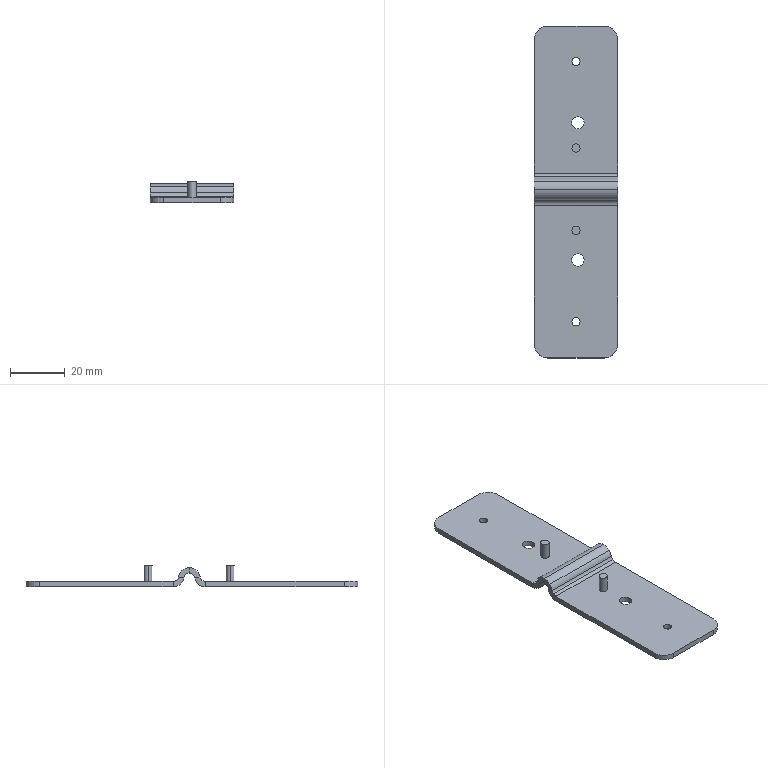Part | NX | features BREP 1 | 1 solid | 48 faces | box 30.5 x 121 x 8 mm | volume 7636 mm3 | cylinder 28 | plane 20 | commonest cylinder face diameters 3 x8 4 x6 8 x6 4.5 x4 10 x4
STEP:
#1=CARTESIAN_POINT('',(94.764,92.,225.465));
#2=VERTEX_POINT('',#1);
#3=CARTESIAN_POINT('',(97.764,92.,225.465));
#4=VERTEX_POINT('',#3);
#5=CARTESIAN_POINT('',(96.264,92.,225.465));
#6=DIRECTION('',(0.,0.,1.));
#7=DIRECTION('',(1.,0.,0.));
#8=AXIS2_PLACEMENT_3D('',#5,#6,#7);
#9=CIRCLE('',#8,1.5);
#10=EDGE_CURVE('',#2,#4,#9,.T.);
#11=ORIENTED_EDGE('',*,*,#10,.T.);
#12=CARTESIAN_POINT('',(96.264,92.,225.465));
#13=DIRECTION('',(0.,0.,1.));
#14=DIRECTION('',(1.,0.,0.));
#15=AXIS2_PLACEMENT_3D('',#12,#13,#14);
#16=CIRCLE('',#15,1.5);
#17=EDGE_CURVE('',#4,#2,#16,.T.);
#18=ORIENTED_EDGE('',*,*,#17,.T.);
#19=EDGE_LOOP('',(#11,#18));
#20=FACE_BOUND('',#19,.T.);
#21=CARTESIAN_POINT('',(0.,0.,225.465));
#22=DIRECTION('',(0.,0.,1.));
#23=DIRECTION('',(1.,0.,0.));
#24=AXIS2_PLACEMENT_3D('',#21,#22,#23);
#25=PLANE('',#24);
#26=ADVANCED_FACE('',(#20),#25,.T.);
#27=CARTESIAN_POINT('',(94.764,92.,219.465));
#28=VERTEX_POINT('',#27);
#29=CARTESIAN_POINT('',(94.764,92.,222.465));
#30=DIRECTION('',(0.,0.,-1.));
#31=VECTOR('',#30,1000.);
#32=LINE('',#29,#31);
#33=EDGE_CURVE('',#2,#28,#32,.T.);
#34=ORIENTED_EDGE('',*,*,#33,.T.);
#35=CARTESIAN_POINT('',(97.764,92.,219.465));
#36=VERTEX_POINT('',#35);
#37=CARTESIAN_POINT('',(96.264,92.,219.465));
#38=DIRECTION('',(0.,0.,1.));
#39=DIRECTION('',(1.,0.,0.));
#40=AXIS2_PLACEMENT_3D('',#37,#38,#39);
#41=CIRCLE('',#40,1.5);
#42=EDGE_CURVE('',#28,#36,#41,.T.);
#43=ORIENTED_EDGE('',*,*,#42,.T.);
#44=CARTESIAN_POINT('',(97.764,92.,222.465));
#45=DIRECTION('',(0.,0.,-1.));
#46=VECTOR('',#45,1000.);
#47=LINE('',#44,#46);
#48=EDGE_CURVE('',#4,#36,#47,.T.);
#49=ORIENTED_EDGE('',*,*,#48,.F.);
#50=ORIENTED_EDGE('',*,*,#10,.F.);
#51=EDGE_LOOP('',(#34,#43,#49,#50));
#52=FACE_BOUND('',#51,.T.);
#53=CARTESIAN_POINT('',(96.264,92.,222.465));
#54=DIRECTION('',(0.,0.,1.));
#55=DIRECTION('',(-1.,0.,0.));
#56=AXIS2_PLACEMENT_3D('',#53,#54,#55);
#57=CYLINDRICAL_SURFACE('',#56,1.5);
#58=ADVANCED_FACE('',(#52),#57,.T.);
#59=ORIENTED_EDGE('',*,*,#48,.T.);
#60=CARTESIAN_POINT('',(96.264,92.,219.465));
#61=DIRECTION('',(0.,0.,1.));
#62=DIRECTION('',(1.,0.,0.));
#63=AXIS2_PLACEMENT_3D('',#60,#61,#62);
#64=CIRCLE('',#63,1.5);
#65=EDGE_CURVE('',#36,#28,#64,.T.);
#66=ORIENTED_EDGE('',*,*,#65,.T.);
#67=ORIENTED_EDGE('',*,*,#33,.F.);
#68=ORIENTED_EDGE('',*,*,#17,.F.);
#69=EDGE_LOOP('',(#59,#66,#67,#68));
#70=FACE_BOUND('',#69,.T.);
#71=CARTESIAN_POINT('',(96.264,92.,222.465));
#72=DIRECTION('',(0.,0.,1.));
#73=DIRECTION('',(-1.,0.,0.));
#74=AXIS2_PLACEMENT_3D('',#71,#72,#73);
#75=CYLINDRICAL_SURFACE('',#74,1.5);
#76=ADVANCED_FACE('',(#70),#75,.T.);
#77=CARTESIAN_POINT('',(94.689,81.216,217.465));
#78=VERTEX_POINT('',#77);
#79=CARTESIAN_POINT('',(94.689,81.216,219.465));
#80=VERTEX_POINT('',#79);
#81=CARTESIAN_POINT('',(94.689,81.216,217.465));
#82=DIRECTION('',(0.,0.,1.));
#83=VECTOR('',#82,1000.);
#84=LINE('',#81,#83);
#85=EDGE_CURVE('',#78,#80,#84,.T.);
#86=ORIENTED_EDGE('',*,*,#85,.T.);
#87=CARTESIAN_POINT('',(99.189,81.216,219.465));
#88=VERTEX_POINT('',#87);
#89=CARTESIAN_POINT('',(96.939,81.216,219.465));
#90=DIRECTION('',(0.,0.,-1.));
#91=DIRECTION('',(1.,0.,0.));
#92=AXIS2_PLACEMENT_3D('',#89,#90,#91);
#93=CIRCLE('',#92,2.25);
#94=EDGE_CURVE('',#88,#80,#93,.T.);
#95=ORIENTED_EDGE('',*,*,#94,.F.);
#96=CARTESIAN_POINT('',(99.189,81.216,217.465));
#97=VERTEX_POINT('',#96);
#98=CARTESIAN_POINT('',(99.189,81.216,217.465));
#99=DIRECTION('',(0.,0.,-1.));
#100=VECTOR('',#99,1000.);
#101=LINE('',#98,#100);
#102=EDGE_CURVE('',#88,#97,#101,.T.);
#103=ORIENTED_EDGE('',*,*,#102,.T.);
#104=CARTESIAN_POINT('',(96.939,81.216,217.465));
#105=DIRECTION('',(0.,0.,1.));
#106=DIRECTION('',(1.,0.,0.));
#107=AXIS2_PLACEMENT_3D('',#104,#105,#106);
#108=CIRCLE('',#107,2.25);
#109=EDGE_CURVE('',#78,#97,#108,.T.);
#110=ORIENTED_EDGE('',*,*,#109,.F.);
#111=EDGE_LOOP('',(#86,#95,#103,#110));
#112=FACE_BOUND('',#111,.T.);
#113=CARTESIAN_POINT('',(96.939,81.216,217.465));
#114=DIRECTION('',(0.,0.,1.));
#115=DIRECTION('',(-1.,0.,0.));
#116=AXIS2_PLACEMENT_3D('',#113,#114,#115);
#117=CYLINDRICAL_SURFACE('',#116,2.25);
#118=ADVANCED_FACE('',(#112),#117,.F.);
#119=ORIENTED_EDGE('',*,*,#102,.F.);
#120=CARTESIAN_POINT('',(96.939,81.216,219.465));
#121=DIRECTION('',(0.,0.,-1.));
#122=DIRECTION('',(1.,0.,0.));
#123=AXIS2_PLACEMENT_3D('',#120,#121,#122);
#124=CIRCLE('',#123,2.25);
#125=EDGE_CURVE('',#80,#88,#124,.T.);
#126=ORIENTED_EDGE('',*,*,#125,.F.);
#127=ORIENTED_EDGE('',*,*,#85,.F.);
#128=CARTESIAN_POINT('',(96.939,81.216,217.465));
#129=DIRECTION('',(0.,0.,1.));
#130=DIRECTION('',(1.,0.,0.));
#131=AXIS2_PLACEMENT_3D('',#128,#129,#130);
#132=CIRCLE('',#131,2.25);
#133=EDGE_CURVE('',#97,#78,#132,.T.);
#134=ORIENTED_EDGE('',*,*,#133,.F.);
#135=EDGE_LOOP('',(#119,#126,#127,#134));
#136=FACE_BOUND('',#135,.T.);
#137=CARTESIAN_POINT('',(96.939,81.216,217.465));
#138=DIRECTION('',(0.,0.,1.));
#139=DIRECTION('',(1.,0.,0.));
#140=AXIS2_PLACEMENT_3D('',#137,#138,#139);
#141=CYLINDRICAL_SURFACE('',#140,2.25);
#142=ADVANCED_FACE('',(#136),#141,.F.);
#143=CARTESIAN_POINT('',(111.514,103.056,221.132));
#144=VERTEX_POINT('',#143);
#145=CARTESIAN_POINT('',(111.514,102.375,219.937));
#146=VERTEX_POINT('',#145);
#147=CARTESIAN_POINT('',(111.514,103.056,221.132));
#148=CARTESIAN_POINT('',(111.514,103.019,220.91));
#149=CARTESIAN_POINT('',(111.514,102.95,220.694));
#150=CARTESIAN_POINT('',(111.514,102.851,220.489));
#151=CARTESIAN_POINT('',(111.514,102.694,220.254));
#152=CARTESIAN_POINT('',(111.514,102.5,220.051));
#153=CARTESIAN_POINT('',(111.514,102.459,220.011));
#154=CARTESIAN_POINT('',(111.514,102.418,219.974));
#155=CARTESIAN_POINT('',(111.514,102.375,219.937));
#156=B_SPLINE_CURVE_WITH_KNOTS('',5,(#147,#148,#149,#150,#151,#152,#153,#154,#155),.UNSPECIFIED.,.F.,.F.,(6,3,6),(0.,0.8,1.),.UNSPECIFIED.);
#157=EDGE_CURVE('',#144,#146,#156,.T.);
#158=ORIENTED_EDGE('',*,*,#157,.T.);
#159=CARTESIAN_POINT('',(111.514,101.084,219.465));
#160=VERTEX_POINT('',#159);
#161=CARTESIAN_POINT('',(111.514,102.375,219.937));
#162=CARTESIAN_POINT('',(111.514,102.203,219.793));
#163=CARTESIAN_POINT('',(111.514,102.012,219.672));
#164=CARTESIAN_POINT('',(111.514,101.804,219.579));
#165=CARTESIAN_POINT('',(111.514,101.532,219.5));
#166=CARTESIAN_POINT('',(111.514,101.252,219.471));
#167=CARTESIAN_POINT('',(111.514,101.196,219.467));
#168=CARTESIAN_POINT('',(111.514,101.14,219.465));
#169=CARTESIAN_POINT('',(111.514,101.084,219.465));
#170=B_SPLINE_CURVE_WITH_KNOTS('',5,(#161,#162,#163,#164,#165,#166,#167,#168,#169),.UNSPECIFIED.,.F.,.F.,(6,3,6),(0.,0.8,1.),.UNSPECIFIED.);
#171=EDGE_CURVE('',#146,#160,#170,.T.);
#172=ORIENTED_EDGE('',*,*,#171,.T.);
#173=CARTESIAN_POINT('',(111.514,101.084,217.465));
#174=VERTEX_POINT('',#173);
#175=CARTESIAN_POINT('',(111.514,101.084,218.465));
#176=DIRECTION('',(0.,0.,-1.));
#177=VECTOR('',#176,1000.);
#178=LINE('',#175,#177);
#179=EDGE_CURVE('',#160,#174,#178,.T.);
#180=ORIENTED_EDGE('',*,*,#179,.T.);
#181=CARTESIAN_POINT('',(111.514,105.028,220.798));
#182=VERTEX_POINT('',#181);
#183=CARTESIAN_POINT('',(111.514,101.084,221.465));
#184=DIRECTION('',(1.,0.,0.));
#185=DIRECTION('',(0.,0.,-1.));
#186=AXIS2_PLACEMENT_3D('',#183,#184,#185);
#187=CIRCLE('',#186,4.);
#188=EDGE_CURVE('',#174,#182,#187,.T.);
#189=ORIENTED_EDGE('',*,*,#188,.T.);
#190=CARTESIAN_POINT('',(111.514,104.042,220.965));
#191=DIRECTION('',(0.,0.986,-0.1667));
#192=VECTOR('',#191,1000.);
#193=LINE('',#190,#192);
#194=EDGE_CURVE('',#144,#182,#193,.T.);
#195=ORIENTED_EDGE('',*,*,#194,.F.);
#196=EDGE_LOOP('',(#158,#172,#180,#189,#195));
#197=FACE_BOUND('',#196,.T.);
#198=CARTESIAN_POINT('',(111.514,101.084,217.465));
#199=DIRECTION('',(1.,0.,0.));
#200=DIRECTION('',(0.,-1.,0.));
#201=AXIS2_PLACEMENT_3D('',#198,#199,#200);
#202=PLANE('',#201);
#203=ADVANCED_FACE('',(#197),#202,.T.);
#204=CARTESIAN_POINT('',(81.014,101.084,219.465));
#205=VERTEX_POINT('',#204);
#206=CARTESIAN_POINT('',(96.264,101.084,219.465));
#207=DIRECTION('',(1.,0.,0.));
#208=VECTOR('',#207,1000.);
#209=LINE('',#206,#208);
#210=EDGE_CURVE('',#205,#160,#209,.T.);
#211=ORIENTED_EDGE('',*,*,#210,.T.);
#212=ORIENTED_EDGE('',*,*,#171,.F.);
#213=CARTESIAN_POINT('',(81.014,102.375,219.937));
#214=VERTEX_POINT('',#213);
#215=CARTESIAN_POINT('',(96.264,102.375,219.937));
#216=DIRECTION('',(-1.,0.,0.));
#217=VECTOR('',#216,1000.);
#218=LINE('',#215,#217);
#219=EDGE_CURVE('',#146,#214,#218,.T.);
#220=ORIENTED_EDGE('',*,*,#219,.T.);
#221=CARTESIAN_POINT('',(81.014,101.084,221.465));
#222=DIRECTION('',(1.,0.,0.));
#223=DIRECTION('',(0.,0.,-1.));
#224=AXIS2_PLACEMENT_3D('',#221,#222,#223);
#225=CIRCLE('',#224,2.);
#226=EDGE_CURVE('',#205,#214,#225,.T.);
#227=ORIENTED_EDGE('',*,*,#226,.F.);
#228=EDGE_LOOP('',(#211,#212,#220,#227));
#229=FACE_BOUND('',#228,.T.);
#230=CARTESIAN_POINT('',(96.264,101.084,221.465));
#231=DIRECTION('',(1.,0.,0.));
#232=DIRECTION('',(0.,-0.6455,0.7638));
#233=AXIS2_PLACEMENT_3D('',#230,#231,#232);
#234=CYLINDRICAL_SURFACE('',#233,2.);
#235=ADVANCED_FACE('',(#229),#234,.F.);
#236=CARTESIAN_POINT('',(81.014,103.056,221.132));
#237=VERTEX_POINT('',#236);
#238=CARTESIAN_POINT('',(96.264,103.056,221.132));
#239=DIRECTION('',(-1.,0.,0.));
#240=VECTOR('',#239,1000.);
#241=LINE('',#238,#240);
#242=EDGE_CURVE('',#144,#237,#241,.T.);
#243=ORIENTED_EDGE('',*,*,#242,.T.);
#244=CARTESIAN_POINT('',(81.014,101.084,221.465));
#245=DIRECTION('',(1.,0.,0.));
#246=DIRECTION('',(0.,0.,-1.));
#247=AXIS2_PLACEMENT_3D('',#244,#245,#246);
#248=CIRCLE('',#247,2.);
#249=EDGE_CURVE('',#214,#237,#248,.T.);
#250=ORIENTED_EDGE('',*,*,#249,.F.);
#251=ORIENTED_EDGE('',*,*,#219,.F.);
#252=ORIENTED_EDGE('',*,*,#157,.F.);
#253=EDGE_LOOP('',(#243,#250,#251,#252));
#254=FACE_BOUND('',#253,.T.);
#255=CARTESIAN_POINT('',(96.264,101.084,221.465));
#256=DIRECTION('',(1.,0.,0.));
#257=DIRECTION('',(0.,0.6455,-0.7638));
#258=AXIS2_PLACEMENT_3D('',#255,#256,#257);
#259=CYLINDRICAL_SURFACE('',#258,2.);
#260=ADVANCED_FACE('',(#254),#259,.F.);
#261=CARTESIAN_POINT('',(81.014,101.084,217.465));
#262=VERTEX_POINT('',#261);
#263=CARTESIAN_POINT('',(81.014,101.084,218.465));
#264=DIRECTION('',(0.,0.000000001,-1.));
#265=VECTOR('',#264,1000.);
#266=LINE('',#263,#265);
#267=EDGE_CURVE('',#205,#262,#266,.T.);
#268=ORIENTED_EDGE('',*,*,#267,.F.);
#269=ORIENTED_EDGE('',*,*,#226,.T.);
#270=ORIENTED_EDGE('',*,*,#249,.T.);
#271=CARTESIAN_POINT('',(81.014,105.028,220.798));
#272=VERTEX_POINT('',#271);
#273=CARTESIAN_POINT('',(81.014,104.042,220.965));
#274=DIRECTION('',(0.,-0.986,0.1667));
#275=VECTOR('',#274,1000.);
#276=LINE('',#273,#275);
#277=EDGE_CURVE('',#272,#237,#276,.T.);
#278=ORIENTED_EDGE('',*,*,#277,.F.);
#279=CARTESIAN_POINT('',(81.014,105.028,220.798));
#280=CARTESIAN_POINT('',(81.014,104.963,220.412));
#281=CARTESIAN_POINT('',(81.014,104.85,220.033));
#282=CARTESIAN_POINT('',(81.014,104.691,219.671));
#283=CARTESIAN_POINT('',(81.014,104.288,218.992));
#284=CARTESIAN_POINT('',(81.014,103.733,218.43));
#285=CARTESIAN_POINT('',(81.014,103.423,218.184));
#286=CARTESIAN_POINT('',(81.014,102.793,217.802));
#287=CARTESIAN_POINT('',(81.014,102.095,217.573));
#288=CARTESIAN_POINT('',(81.014,101.762,217.501));
#289=CARTESIAN_POINT('',(81.014,101.423,217.465));
#290=CARTESIAN_POINT('',(81.014,101.084,217.465));
#291=B_SPLINE_CURVE_WITH_KNOTS('',5,(#279,#280,#281,#282,#283,#284,#285,#286,#287,#288,#289,#290),.UNSPECIFIED.,.F.,.F.,(6,3,3,6),(0.,0.3491,0.6982,1.),.UNSPECIFIED.);
#292=EDGE_CURVE('',#272,#262,#291,.T.);
#293=ORIENTED_EDGE('',*,*,#292,.T.);
#294=EDGE_LOOP('',(#268,#269,#270,#278,#293));
#295=FACE_BOUND('',#294,.T.);
#296=CARTESIAN_POINT('',(81.014,101.084,217.465));
#297=DIRECTION('',(1.,0.,0.));
#298=DIRECTION('',(0.,-1.,0.));
#299=AXIS2_PLACEMENT_3D('',#296,#297,#298);
#300=PLANE('',#299);
#301=ADVANCED_FACE('',(#295),#300,.F.);
#302=ORIENTED_EDGE('',*,*,#292,.F.);
#303=CARTESIAN_POINT('',(96.264,105.028,220.798));
#304=DIRECTION('',(-1.,0.,0.));
#305=VECTOR('',#304,1000.);
#306=LINE('',#303,#305);
#307=EDGE_CURVE('',#182,#272,#306,.T.);
#308=ORIENTED_EDGE('',*,*,#307,.F.);
#309=ORIENTED_EDGE('',*,*,#188,.F.);
#310=CARTESIAN_POINT('',(96.264,101.084,217.465));
#311=DIRECTION('',(-1.,0.,0.));
#312=VECTOR('',#311,1000.);
#313=LINE('',#310,#312);
#314=EDGE_CURVE('',#174,#262,#313,.T.);
#315=ORIENTED_EDGE('',*,*,#314,.T.);
#316=EDGE_LOOP('',(#302,#308,#309,#315));
#317=FACE_BOUND('',#316,.T.);
#318=CARTESIAN_POINT('',(96.264,101.084,221.465));
#319=DIRECTION('',(1.,0.,0.));
#320=DIRECTION('',(0.,0.,-1.));
#321=AXIS2_PLACEMENT_3D('',#318,#319,#320);
#322=CYLINDRICAL_SURFACE('',#321,4.);
#323=ADVANCED_FACE('',(#317),#322,.T.);
#324=CARTESIAN_POINT('',(94.764,58.716,217.465));
#325=VERTEX_POINT('',#324);
#326=CARTESIAN_POINT('',(94.764,58.716,219.465));
#327=VERTEX_POINT('',#326);
#328=CARTESIAN_POINT('',(94.764,58.716,217.465));
#329=DIRECTION('',(0.,0.,1.));
#330=VECTOR('',#329,1000.);
#331=LINE('',#328,#330);
#332=EDGE_CURVE('',#325,#327,#331,.T.);
#333=ORIENTED_EDGE('',*,*,#332,.T.);
#334=CARTESIAN_POINT('',(97.764,58.716,219.465));
#335=VERTEX_POINT('',#334);
#336=CARTESIAN_POINT('',(96.264,58.716,219.465));
#337=DIRECTION('',(0.,0.,-1.));
#338=DIRECTION('',(1.,0.,0.));
#339=AXIS2_PLACEMENT_3D('',#336,#337,#338);
#340=CIRCLE('',#339,1.5);
#341=EDGE_CURVE('',#335,#327,#340,.T.);
#342=ORIENTED_EDGE('',*,*,#341,.F.);
#343=CARTESIAN_POINT('',(97.764,58.716,217.465));
#344=VERTEX_POINT('',#343);
#345=CARTESIAN_POINT('',(97.764,58.716,217.465));
#346=DIRECTION('',(0.,0.,-1.));
#347=VECTOR('',#346,1000.);
#348=LINE('',#345,#347);
#349=EDGE_CURVE('',#335,#344,#348,.T.);
#350=ORIENTED_EDGE('',*,*,#349,.T.);
#351=CARTESIAN_POINT('',(96.264,58.716,217.465));
#352=DIRECTION('',(0.,0.,1.));
#353=DIRECTION('',(1.,0.,0.));
#354=AXIS2_PLACEMENT_3D('',#351,#352,#353);
#355=CIRCLE('',#354,1.5);
#356=EDGE_CURVE('',#325,#344,#355,.T.);
#357=ORIENTED_EDGE('',*,*,#356,.F.);
#358=EDGE_LOOP('',(#333,#342,#350,#357));
#359=FACE_BOUND('',#358,.T.);
#360=CARTESIAN_POINT('',(96.264,58.716,217.465));
#361=DIRECTION('',(0.,0.,1.));
#362=DIRECTION('',(-1.,0.,0.));
#363=AXIS2_PLACEMENT_3D('',#360,#361,#362);
#364=CYLINDRICAL_SURFACE('',#363,1.5);
#365=ADVANCED_FACE('',(#359),#364,.F.);
#366=ORIENTED_EDGE('',*,*,#349,.F.);
#367=CARTESIAN_POINT('',(96.264,58.716,219.465));
#368=DIRECTION('',(0.,0.,-1.));
#369=DIRECTION('',(1.,0.,0.));
#370=AXIS2_PLACEMENT_3D('',#367,#368,#369);
#371=CIRCLE('',#370,1.5);
#372=EDGE_CURVE('',#327,#335,#371,.T.);
#373=ORIENTED_EDGE('',*,*,#372,.F.);
#374=ORIENTED_EDGE('',*,*,#332,.F.);
#375=CARTESIAN_POINT('',(96.264,58.716,217.465));
#376=DIRECTION('',(0.,0.,1.));
#377=DIRECTION('',(1.,0.,0.));
#378=AXIS2_PLACEMENT_3D('',#375,#376,#377);
#379=CIRCLE('',#378,1.5);
#380=EDGE_CURVE('',#344,#325,#379,.T.);
#381=ORIENTED_EDGE('',*,*,#380,.F.);
#382=EDGE_LOOP('',(#366,#373,#374,#381));
#383=FACE_BOUND('',#382,.T.);
#384=CARTESIAN_POINT('',(96.264,58.716,217.465));
#385=DIRECTION('',(0.,0.,1.));
#386=DIRECTION('',(1.,0.,0.));
#387=AXIS2_PLACEMENT_3D('',#384,#385,#386);
#388=CYLINDRICAL_SURFACE('',#387,1.5);
#389=ADVANCED_FACE('',(#383),#388,.F.);
#390=CARTESIAN_POINT('',(81.014,104.172,223.293));
#391=VERTEX_POINT('',#390);
#392=CARTESIAN_POINT('',(81.014,107.,220.465));
#393=DIRECTION('',(-1.,0.,0.));
#394=DIRECTION('',(0.,0.,1.));
#395=AXIS2_PLACEMENT_3D('',#392,#393,#394);
#396=CIRCLE('',#395,4.);
#397=EDGE_CURVE('',#237,#391,#396,.T.);
#398=ORIENTED_EDGE('',*,*,#397,.F.);
#399=ORIENTED_EDGE('',*,*,#242,.F.);
#400=CARTESIAN_POINT('',(111.514,104.172,223.293));
#401=VERTEX_POINT('',#400);
#402=CARTESIAN_POINT('',(111.514,107.,220.465));
#403=DIRECTION('',(1.,0.,0.));
#404=DIRECTION('',(0.,0.,1.));
#405=AXIS2_PLACEMENT_3D('',#402,#403,#404);
#406=CIRCLE('',#405,4.);
#407=EDGE_CURVE('',#401,#144,#406,.T.);
#408=ORIENTED_EDGE('',*,*,#407,.F.);
#409=CARTESIAN_POINT('',(95.714,104.172,223.293));
#410=DIRECTION('',(1.,0.,0.));
#411=VECTOR('',#410,1000.);
#412=LINE('',#409,#411);
#413=EDGE_CURVE('',#391,#401,#412,.T.);
#414=ORIENTED_EDGE('',*,*,#413,.F.);
#415=EDGE_LOOP('',(#398,#399,#408,#414));
#416=FACE_BOUND('',#415,.T.);
#417=CARTESIAN_POINT('',(95.714,107.,220.465));
#418=DIRECTION('',(-1.,0.,0.));
#419=DIRECTION('',(0.,0.7071,-0.7071));
#420=AXIS2_PLACEMENT_3D('',#417,#418,#419);
#421=CYLINDRICAL_SURFACE('',#420,4.);
#422=ADVANCED_FACE('',(#416),#421,.T.);
#423=CARTESIAN_POINT('',(111.514,107.,224.465));
#424=VERTEX_POINT('',#423);
#425=CARTESIAN_POINT('',(111.514,107.,220.465));
#426=DIRECTION('',(1.,0.,0.));
#427=DIRECTION('',(0.,0.,1.));
#428=AXIS2_PLACEMENT_3D('',#425,#426,#427);
#429=CIRCLE('',#428,4.);
#430=EDGE_CURVE('',#424,#401,#429,.T.);
#431=ORIENTED_EDGE('',*,*,#430,.F.);
#432=CARTESIAN_POINT('',(81.014,107.,224.465));
#433=VERTEX_POINT('',#432);
#434=CARTESIAN_POINT('',(95.714,107.,224.465));
#435=DIRECTION('',(-1.,0.,0.));
#436=VECTOR('',#435,1000.);
#437=LINE('',#434,#436);
#438=EDGE_CURVE('',#424,#433,#437,.T.);
#439=ORIENTED_EDGE('',*,*,#438,.T.);
#440=CARTESIAN_POINT('',(81.014,107.,220.465));
#441=DIRECTION('',(-1.,0.,0.));
#442=DIRECTION('',(0.,0.,1.));
#443=AXIS2_PLACEMENT_3D('',#440,#441,#442);
#444=CIRCLE('',#443,4.);
#445=EDGE_CURVE('',#391,#433,#444,.T.);
#446=ORIENTED_EDGE('',*,*,#445,.F.);
#447=ORIENTED_EDGE('',*,*,#413,.T.);
#448=EDGE_LOOP('',(#431,#439,#446,#447));
#449=FACE_BOUND('',#448,.T.);
#450=CARTESIAN_POINT('',(95.714,107.,220.465));
#451=DIRECTION('',(-1.,0.,0.));
#452=DIRECTION('',(0.,-0.7071,0.7071));
#453=AXIS2_PLACEMENT_3D('',#450,#451,#452);
#454=CYLINDRICAL_SURFACE('',#453,4.);
#455=ADVANCED_FACE('',(#449),#454,.T.);
#456=ORIENTED_EDGE('',*,*,#307,.T.);
#457=CARTESIAN_POINT('',(81.014,107.,222.465));
#458=VERTEX_POINT('',#457);
#459=CARTESIAN_POINT('',(81.014,107.,220.465));
#460=DIRECTION('',(1.,0.,0.));
#461=DIRECTION('',(0.,0.,1.));
#462=AXIS2_PLACEMENT_3D('',#459,#460,#461);
#463=CIRCLE('',#462,2.);
#464=EDGE_CURVE('',#458,#272,#463,.T.);
#465=ORIENTED_EDGE('',*,*,#464,.F.);
#466=CARTESIAN_POINT('',(111.514,107.,222.465));
#467=VERTEX_POINT('',#466);
#468=CARTESIAN_POINT('',(95.714,107.,222.465));
#469=DIRECTION('',(-1.,0.,0.));
#470=VECTOR('',#469,1000.);
#471=LINE('',#468,#470);
#472=EDGE_CURVE('',#467,#458,#471,.T.);
#473=ORIENTED_EDGE('',*,*,#472,.F.);
#474=CARTESIAN_POINT('',(111.514,107.,220.465));
#475=DIRECTION('',(-1.,0.,0.));
#476=DIRECTION('',(0.,0.,1.));
#477=AXIS2_PLACEMENT_3D('',#474,#475,#476);
#478=CIRCLE('',#477,2.);
#479=EDGE_CURVE('',#182,#467,#478,.T.);
#480=ORIENTED_EDGE('',*,*,#479,.F.);
#481=EDGE_LOOP('',(#456,#465,#473,#480));
#482=FACE_BOUND('',#481,.T.);
#483=CARTESIAN_POINT('',(95.714,107.,220.465));
#484=DIRECTION('',(-1.,0.,0.));
#485=DIRECTION('',(0.,-1.,0.));
#486=AXIS2_PLACEMENT_3D('',#483,#484,#485);
#487=CYLINDRICAL_SURFACE('',#486,2.);
#488=ADVANCED_FACE('',(#482),#487,.F.);
#489=ORIENTED_EDGE('',*,*,#430,.T.);
#490=ORIENTED_EDGE('',*,*,#407,.T.);
#491=ORIENTED_EDGE('',*,*,#194,.T.);
#492=ORIENTED_EDGE('',*,*,#479,.T.);
#493=CARTESIAN_POINT('',(111.514,107.,223.465));
#494=DIRECTION('',(0.,0.,-1.));
#495=VECTOR('',#494,1000.);
#496=LINE('',#493,#495);
#497=EDGE_CURVE('',#424,#467,#496,.T.);
#498=ORIENTED_EDGE('',*,*,#497,.F.);
#499=EDGE_LOOP('',(#489,#490,#491,#492,#498));
#500=FACE_BOUND('',#499,.T.);
#501=CARTESIAN_POINT('',(111.514,105.028,220.798));
#502=DIRECTION('',(-1.,0.,0.));
#503=DIRECTION('',(0.,0.,-1.));
#504=AXIS2_PLACEMENT_3D('',#501,#502,#503);
#505=PLANE('',#504);
#506=ADVANCED_FACE('',(#500),#505,.F.);
#507=CARTESIAN_POINT('',(81.014,109.828,223.293));
#508=VERTEX_POINT('',#507);
#509=CARTESIAN_POINT('',(81.014,107.,220.465));
#510=DIRECTION('',(-1.,0.,0.));
#511=DIRECTION('',(0.,0.,-1.));
#512=AXIS2_PLACEMENT_3D('',#509,#510,#511);
#513=CIRCLE('',#512,4.);
#514=EDGE_CURVE('',#433,#508,#513,.T.);
#515=ORIENTED_EDGE('',*,*,#514,.F.);
#516=ORIENTED_EDGE('',*,*,#438,.F.);
#517=CARTESIAN_POINT('',(111.514,109.828,223.293));
#518=VERTEX_POINT('',#517);
#519=CARTESIAN_POINT('',(111.514,107.,220.465));
#520=DIRECTION('',(1.,0.,0.));
#521=DIRECTION('',(0.,0.,-1.));
#522=AXIS2_PLACEMENT_3D('',#519,#520,#521);
#523=CIRCLE('',#522,4.);
#524=EDGE_CURVE('',#518,#424,#523,.T.);
#525=ORIENTED_EDGE('',*,*,#524,.F.);
#526=CARTESIAN_POINT('',(95.714,109.828,223.293));
#527=DIRECTION('',(-1.,0.,0.));
#528=VECTOR('',#527,1000.);
#529=LINE('',#526,#528);
#530=EDGE_CURVE('',#518,#508,#529,.T.);
#531=ORIENTED_EDGE('',*,*,#530,.T.);
#532=EDGE_LOOP('',(#515,#516,#525,#531));
#533=FACE_BOUND('',#532,.T.);
#534=CARTESIAN_POINT('',(95.714,107.,220.465));
#535=DIRECTION('',(1.,0.,0.));
#536=DIRECTION('',(0.,0.7071,0.7071));
#537=AXIS2_PLACEMENT_3D('',#534,#535,#536);
#538=CYLINDRICAL_SURFACE('',#537,4.);
#539=ADVANCED_FACE('',(#533),#538,.T.);
#540=ORIENTED_EDGE('',*,*,#277,.T.);
#541=ORIENTED_EDGE('',*,*,#397,.T.);
#542=ORIENTED_EDGE('',*,*,#445,.T.);
#543=CARTESIAN_POINT('',(81.014,107.,223.465));
#544=DIRECTION('',(0.,0.,-1.));
#545=VECTOR('',#544,1000.);
#546=LINE('',#543,#545);
#547=EDGE_CURVE('',#433,#458,#546,.T.);
#548=ORIENTED_EDGE('',*,*,#547,.T.);
#549=ORIENTED_EDGE('',*,*,#464,.T.);
#550=EDGE_LOOP('',(#540,#541,#542,#548,#549));
#551=FACE_BOUND('',#550,.T.);
#552=CARTESIAN_POINT('',(81.014,107.,222.465));
#553=DIRECTION('',(1.,0.,0.));
#554=DIRECTION('',(0.,-1.,0.));
#555=AXIS2_PLACEMENT_3D('',#552,#553,#554);
#556=PLANE('',#555);
#557=ADVANCED_FACE('',(#551),#556,.F.);
#558=CARTESIAN_POINT('',(111.514,108.972,220.798));
#559=VERTEX_POINT('',#558);
#560=CARTESIAN_POINT('',(111.514,107.,220.465));
#561=DIRECTION('',(-1.,0.,0.));
#562=DIRECTION('',(0.,0.,-1.));
#563=AXIS2_PLACEMENT_3D('',#560,#561,#562);
#564=CIRCLE('',#563,2.);
#565=EDGE_CURVE('',#467,#559,#564,.T.);
#566=ORIENTED_EDGE('',*,*,#565,.F.);
#567=ORIENTED_EDGE('',*,*,#472,.T.);
#568=CARTESIAN_POINT('',(81.014,108.972,220.798));
#569=VERTEX_POINT('',#568);
#570=CARTESIAN_POINT('',(81.014,107.,220.465));
#571=DIRECTION('',(1.,0.,0.));
#572=DIRECTION('',(0.,0.,-1.));
#573=AXIS2_PLACEMENT_3D('',#570,#571,#572);
#574=CIRCLE('',#573,2.);
#575=EDGE_CURVE('',#569,#458,#574,.T.);
#576=ORIENTED_EDGE('',*,*,#575,.F.);
#577=CARTESIAN_POINT('',(95.714,108.972,220.798));
#578=DIRECTION('',(1.,0.,0.));
#579=VECTOR('',#578,1000.);
#580=LINE('',#577,#579);
#581=EDGE_CURVE('',#569,#559,#580,.T.);
#582=ORIENTED_EDGE('',*,*,#581,.T.);
#583=EDGE_LOOP('',(#566,#567,#576,#582));
#584=FACE_BOUND('',#583,.T.);
#585=CARTESIAN_POINT('',(95.714,107.,220.465));
#586=DIRECTION('',(1.,0.,0.));
#587=DIRECTION('',(0.,1.,0.));
#588=AXIS2_PLACEMENT_3D('',#585,#586,#587);
#589=CYLINDRICAL_SURFACE('',#588,2.);
#590=ADVANCED_FACE('',(#584),#589,.F.);
#591=CARTESIAN_POINT('',(111.514,110.944,221.132));
#592=VERTEX_POINT('',#591);
#593=CARTESIAN_POINT('',(111.514,107.,220.465));
#594=DIRECTION('',(1.,0.,0.));
#595=DIRECTION('',(0.,0.,-1.));
#596=AXIS2_PLACEMENT_3D('',#593,#594,#595);
#597=CIRCLE('',#596,4.);
#598=EDGE_CURVE('',#592,#518,#597,.T.);
#599=ORIENTED_EDGE('',*,*,#598,.F.);
#600=CARTESIAN_POINT('',(81.014,110.944,221.132));
#601=VERTEX_POINT('',#600);
#602=CARTESIAN_POINT('',(95.714,110.944,221.132));
#603=DIRECTION('',(1.,0.,0.));
#604=VECTOR('',#603,1000.);
#605=LINE('',#602,#604);
#606=EDGE_CURVE('',#601,#592,#605,.T.);
#607=ORIENTED_EDGE('',*,*,#606,.F.);
#608=CARTESIAN_POINT('',(81.014,107.,220.465));
#609=DIRECTION('',(-1.,0.,0.));
#610=DIRECTION('',(0.,0.,-1.));
#611=AXIS2_PLACEMENT_3D('',#608,#609,#610);
#612=CIRCLE('',#611,4.);
#613=EDGE_CURVE('',#508,#601,#612,.T.);
#614=ORIENTED_EDGE('',*,*,#613,.F.);
#615=ORIENTED_EDGE('',*,*,#530,.F.);
#616=EDGE_LOOP('',(#599,#607,#614,#615));
#617=FACE_BOUND('',#616,.T.);
#618=CARTESIAN_POINT('',(95.714,107.,220.465));
#619=DIRECTION('',(1.,0.,0.));
#620=DIRECTION('',(0.,-0.7071,-0.7071));
#621=AXIS2_PLACEMENT_3D('',#618,#619,#620);
#622=CYLINDRICAL_SURFACE('',#621,4.);
#623=ADVANCED_FACE('',(#617),#622,.T.);
#624=CARTESIAN_POINT('',(111.514,109.958,220.965));
#625=DIRECTION('',(0.,0.986,0.1667));
#626=VECTOR('',#625,1000.);
#627=LINE('',#624,#626);
#628=EDGE_CURVE('',#559,#592,#627,.T.);
#629=ORIENTED_EDGE('',*,*,#628,.T.);
#630=ORIENTED_EDGE('',*,*,#598,.T.);
#631=ORIENTED_EDGE('',*,*,#524,.T.);
#632=ORIENTED_EDGE('',*,*,#497,.T.);
#633=ORIENTED_EDGE('',*,*,#565,.T.);
#634=EDGE_LOOP('',(#629,#630,#631,#632,#633));
#635=FACE_BOUND('',#634,.T.);
#636=CARTESIAN_POINT('',(111.514,107.,222.465));
#637=DIRECTION('',(-1.,0.,0.));
#638=DIRECTION('',(0.,0.,-1.));
#639=AXIS2_PLACEMENT_3D('',#636,#637,#638);
#640=PLANE('',#639);
#641=ADVANCED_FACE('',(#635),#640,.F.);
#642=ORIENTED_EDGE('',*,*,#514,.T.);
#643=ORIENTED_EDGE('',*,*,#613,.T.);
#644=CARTESIAN_POINT('',(81.014,109.958,220.965));
#645=DIRECTION('',(0.,-0.986,-0.1667));
#646=VECTOR('',#645,1000.);
#647=LINE('',#644,#646);
#648=EDGE_CURVE('',#601,#569,#647,.T.);
#649=ORIENTED_EDGE('',*,*,#648,.T.);
#650=ORIENTED_EDGE('',*,*,#575,.T.);
#651=ORIENTED_EDGE('',*,*,#547,.F.);
#652=EDGE_LOOP('',(#642,#643,#649,#650,#651));
#653=FACE_BOUND('',#652,.T.);
#654=CARTESIAN_POINT('',(81.014,108.972,220.798));
#655=DIRECTION('',(1.,0.,0.));
#656=DIRECTION('',(0.,-1.,0.));
#657=AXIS2_PLACEMENT_3D('',#654,#655,#656);
#658=PLANE('',#657);
#659=ADVANCED_FACE('',(#653),#658,.F.);
#660=CARTESIAN_POINT('',(111.514,112.916,217.465));
#661=VERTEX_POINT('',#660);
#662=CARTESIAN_POINT('',(111.514,112.916,221.465));
#663=DIRECTION('',(1.,0.,0.));
#664=DIRECTION('',(0.,0.,1.));
#665=AXIS2_PLACEMENT_3D('',#662,#663,#664);
#666=CIRCLE('',#665,4.);
#667=EDGE_CURVE('',#559,#661,#666,.T.);
#668=ORIENTED_EDGE('',*,*,#667,.F.);
#669=ORIENTED_EDGE('',*,*,#581,.F.);
#670=CARTESIAN_POINT('',(81.014,112.916,217.465));
#671=VERTEX_POINT('',#670);
#672=CARTESIAN_POINT('',(81.014,112.916,221.465));
#673=DIRECTION('',(-1.,0.,0.));
#674=DIRECTION('',(0.,0.,1.));
#675=AXIS2_PLACEMENT_3D('',#672,#673,#674);
#676=CIRCLE('',#675,4.);
#677=EDGE_CURVE('',#671,#569,#676,.T.);
#678=ORIENTED_EDGE('',*,*,#677,.F.);
#679=CARTESIAN_POINT('',(96.264,112.916,217.465));
#680=DIRECTION('',(1.,0.,0.));
#681=VECTOR('',#680,1000.);
#682=LINE('',#679,#681);
#683=EDGE_CURVE('',#671,#661,#682,.T.);
#684=ORIENTED_EDGE('',*,*,#683,.T.);
#685=EDGE_LOOP('',(#668,#669,#678,#684));
#686=FACE_BOUND('',#685,.T.);
#687=CARTESIAN_POINT('',(96.264,112.916,221.465));
#688=DIRECTION('',(-1.,0.,0.));
#689=DIRECTION('',(0.,0.,-1.));
#690=AXIS2_PLACEMENT_3D('',#687,#688,#689);
#691=CYLINDRICAL_SURFACE('',#690,4.);
#692=ADVANCED_FACE('',(#686),#691,.T.);
#693=CARTESIAN_POINT('',(111.514,111.625,219.937));
#694=VERTEX_POINT('',#693);
#695=CARTESIAN_POINT('',(111.514,112.916,221.465));
#696=DIRECTION('',(-1.,0.,0.));
#697=DIRECTION('',(0.,0.,1.));
#698=AXIS2_PLACEMENT_3D('',#695,#696,#697);
#699=CIRCLE('',#698,2.);
#700=EDGE_CURVE('',#694,#592,#699,.T.);
#701=ORIENTED_EDGE('',*,*,#700,.F.);
#702=CARTESIAN_POINT('',(81.014,111.625,219.937));
#703=VERTEX_POINT('',#702);
#704=CARTESIAN_POINT('',(96.264,111.625,219.937));
#705=DIRECTION('',(1.,0.,0.));
#706=VECTOR('',#705,1000.);
#707=LINE('',#704,#706);
#708=EDGE_CURVE('',#703,#694,#707,.T.);
#709=ORIENTED_EDGE('',*,*,#708,.F.);
#710=CARTESIAN_POINT('',(81.014,112.916,221.465));
#711=DIRECTION('',(1.,0.,0.));
#712=DIRECTION('',(0.,0.,1.));
#713=AXIS2_PLACEMENT_3D('',#710,#711,#712);
#714=CIRCLE('',#713,2.);
#715=EDGE_CURVE('',#601,#703,#714,.T.);
#716=ORIENTED_EDGE('',*,*,#715,.F.);
#717=ORIENTED_EDGE('',*,*,#606,.T.);
#718=EDGE_LOOP('',(#701,#709,#716,#717));
#719=FACE_BOUND('',#718,.T.);
#720=CARTESIAN_POINT('',(96.264,112.916,221.465));
#721=DIRECTION('',(-1.,0.,0.));
#722=DIRECTION('',(0.,-0.6455,-0.7638));
#723=AXIS2_PLACEMENT_3D('',#720,#721,#722);
#724=CYLINDRICAL_SURFACE('',#723,2.);
#725=ADVANCED_FACE('',(#719),#724,.F.);
#726=CARTESIAN_POINT('',(111.514,112.916,219.465));
#727=VERTEX_POINT('',#726);
#728=CARTESIAN_POINT('',(111.514,112.916,221.465));
#729=DIRECTION('',(-1.,0.,0.));
#730=DIRECTION('',(0.,0.,1.));
#731=AXIS2_PLACEMENT_3D('',#728,#729,#730);
#732=CIRCLE('',#731,2.);
#733=EDGE_CURVE('',#727,#694,#732,.T.);
#734=ORIENTED_EDGE('',*,*,#733,.T.);
#735=ORIENTED_EDGE('',*,*,#700,.T.);
#736=ORIENTED_EDGE('',*,*,#628,.F.);
#737=ORIENTED_EDGE('',*,*,#667,.T.);
#738=CARTESIAN_POINT('',(111.514,112.916,218.465));
#739=DIRECTION('',(0.,-0.000000001,-1.));
#740=VECTOR('',#739,1000.);
#741=LINE('',#738,#740);
#742=EDGE_CURVE('',#727,#661,#741,.T.);
#743=ORIENTED_EDGE('',*,*,#742,.F.);
#744=EDGE_LOOP('',(#734,#735,#736,#737,#743));
#745=FACE_BOUND('',#744,.T.);
#746=CARTESIAN_POINT('',(111.514,112.916,217.465));
#747=DIRECTION('',(-1.,0.,0.));
#748=DIRECTION('',(0.,0.,-1.));
#749=AXIS2_PLACEMENT_3D('',#746,#747,#748);
#750=PLANE('',#749);
#751=ADVANCED_FACE('',(#745),#750,.F.);
#752=ORIENTED_EDGE('',*,*,#715,.T.);
#753=CARTESIAN_POINT('',(81.014,112.916,219.465));
#754=VERTEX_POINT('',#753);
#755=CARTESIAN_POINT('',(81.014,111.625,219.937));
#756=CARTESIAN_POINT('',(81.014,111.797,219.793));
#757=CARTESIAN_POINT('',(81.014,111.988,219.672));
#758=CARTESIAN_POINT('',(81.014,112.196,219.579));
#759=CARTESIAN_POINT('',(81.014,112.468,219.5));
#760=CARTESIAN_POINT('',(81.014,112.748,219.471));
#761=CARTESIAN_POINT('',(81.014,112.804,219.467));
#762=CARTESIAN_POINT('',(81.014,112.86,219.465));
#763=CARTESIAN_POINT('',(81.014,112.916,219.465));
#764=B_SPLINE_CURVE_WITH_KNOTS('',5,(#755,#756,#757,#758,#759,#760,#761,#762,#763),.UNSPECIFIED.,.F.,.F.,(6,3,6),(0.,0.8001,1.),.UNSPECIFIED.);
#765=EDGE_CURVE('',#703,#754,#764,.T.);
#766=ORIENTED_EDGE('',*,*,#765,.T.);
#767=CARTESIAN_POINT('',(81.014,112.916,218.465));
#768=DIRECTION('',(0.,0.,-1.));
#769=VECTOR('',#768,1000.);
#770=LINE('',#767,#769);
#771=EDGE_CURVE('',#754,#671,#770,.T.);
#772=ORIENTED_EDGE('',*,*,#771,.T.);
#773=ORIENTED_EDGE('',*,*,#677,.T.);
#774=ORIENTED_EDGE('',*,*,#648,.F.);
#775=EDGE_LOOP('',(#752,#766,#772,#773,#774));
#776=FACE_BOUND('',#775,.T.);
#777=CARTESIAN_POINT('',(81.014,112.916,217.465));
#778=DIRECTION('',(-1.,0.,0.));
#779=DIRECTION('',(0.,0.,-1.));
#780=AXIS2_PLACEMENT_3D('',#777,#778,#779);
#781=PLANE('',#780);
#782=ADVANCED_FACE('',(#776),#781,.T.);
#783=CARTESIAN_POINT('',(99.189,131.216,217.465));
#784=VERTEX_POINT('',#783);
#785=CARTESIAN_POINT('',(94.689,131.216,217.465));
#786=VERTEX_POINT('',#785);
#787=CARTESIAN_POINT('',(96.939,131.216,217.465));
#788=DIRECTION('',(0.,0.,1.));
#789=DIRECTION('',(1.,0.,0.));
#790=AXIS2_PLACEMENT_3D('',#787,#788,#789);
#791=CIRCLE('',#790,2.25);
#792=EDGE_CURVE('',#784,#786,#791,.T.);
#793=ORIENTED_EDGE('',*,*,#792,.F.);
#794=CARTESIAN_POINT('',(99.189,131.216,219.465));
#795=VERTEX_POINT('',#794);
#796=CARTESIAN_POINT('',(99.189,131.216,209.465));
#797=DIRECTION('',(0.,0.,-1.));
#798=VECTOR('',#797,1000.);
#799=LINE('',#796,#798);
#800=EDGE_CURVE('',#795,#784,#799,.T.);
#801=ORIENTED_EDGE('',*,*,#800,.F.);
#802=CARTESIAN_POINT('',(94.689,131.216,219.465));
#803=VERTEX_POINT('',#802);
#804=CARTESIAN_POINT('',(96.939,131.216,219.465));
#805=DIRECTION('',(0.,0.,1.));
#806=DIRECTION('',(1.,0.,0.));
#807=AXIS2_PLACEMENT_3D('',#804,#805,#806);
#808=CIRCLE('',#807,2.25);
#809=EDGE_CURVE('',#795,#803,#808,.T.);
#810=ORIENTED_EDGE('',*,*,#809,.T.);
#811=CARTESIAN_POINT('',(94.689,131.216,209.465));
#812=DIRECTION('',(0.,0.,-1.));
#813=VECTOR('',#812,1000.);
#814=LINE('',#811,#813);
#815=EDGE_CURVE('',#803,#786,#814,.T.);
#816=ORIENTED_EDGE('',*,*,#815,.T.);
#817=EDGE_LOOP('',(#793,#801,#810,#816));
#818=FACE_BOUND('',#817,.T.);
#819=CARTESIAN_POINT('',(96.939,131.216,209.465));
#820=DIRECTION('',(0.,0.,1.));
#821=DIRECTION('',(1.,0.,0.));
#822=AXIS2_PLACEMENT_3D('',#819,#820,#821);
#823=CYLINDRICAL_SURFACE('',#822,2.25);
#824=ADVANCED_FACE('',(#818),#823,.F.);
#825=CARTESIAN_POINT('',(96.939,131.216,217.465));
#826=DIRECTION('',(0.,0.,1.));
#827=DIRECTION('',(1.,0.,0.));
#828=AXIS2_PLACEMENT_3D('',#825,#826,#827);
#829=CIRCLE('',#828,2.25);
#830=EDGE_CURVE('',#786,#784,#829,.T.);
#831=ORIENTED_EDGE('',*,*,#830,.F.);
#832=ORIENTED_EDGE('',*,*,#815,.F.);
#833=CARTESIAN_POINT('',(96.939,131.216,219.465));
#834=DIRECTION('',(0.,0.,1.));
#835=DIRECTION('',(1.,0.,0.));
#836=AXIS2_PLACEMENT_3D('',#833,#834,#835);
#837=CIRCLE('',#836,2.25);
#838=EDGE_CURVE('',#803,#795,#837,.T.);
#839=ORIENTED_EDGE('',*,*,#838,.T.);
#840=ORIENTED_EDGE('',*,*,#800,.T.);
#841=EDGE_LOOP('',(#831,#832,#839,#840));
#842=FACE_BOUND('',#841,.T.);
#843=CARTESIAN_POINT('',(96.939,131.216,209.465));
#844=DIRECTION('',(0.,0.,1.));
#845=DIRECTION('',(1.,0.,0.));
#846=AXIS2_PLACEMENT_3D('',#843,#844,#845);
#847=CYLINDRICAL_SURFACE('',#846,2.25);
#848=ADVANCED_FACE('',(#842),#847,.F.);
#849=CARTESIAN_POINT('',(94.764,153.582,217.465));
#850=VERTEX_POINT('',#849);
#851=CARTESIAN_POINT('',(94.764,153.582,219.465));
#852=VERTEX_POINT('',#851);
#853=CARTESIAN_POINT('',(94.764,153.582,217.465));
#854=DIRECTION('',(0.,0.,1.));
#855=VECTOR('',#854,1000.);
#856=LINE('',#853,#855);
#857=EDGE_CURVE('',#850,#852,#856,.T.);
#858=ORIENTED_EDGE('',*,*,#857,.T.);
#859=CARTESIAN_POINT('',(97.764,153.582,219.465));
#860=VERTEX_POINT('',#859);
#861=CARTESIAN_POINT('',(96.264,153.582,219.465));
#862=DIRECTION('',(0.,0.,-1.));
#863=DIRECTION('',(1.,0.,0.));
#864=AXIS2_PLACEMENT_3D('',#861,#862,#863);
#865=CIRCLE('',#864,1.5);
#866=EDGE_CURVE('',#860,#852,#865,.T.);
#867=ORIENTED_EDGE('',*,*,#866,.F.);
#868=CARTESIAN_POINT('',(97.764,153.582,217.465));
#869=VERTEX_POINT('',#868);
#870=CARTESIAN_POINT('',(97.764,153.582,217.465));
#871=DIRECTION('',(0.,0.,-1.));
#872=VECTOR('',#871,1000.);
#873=LINE('',#870,#872);
#874=EDGE_CURVE('',#860,#869,#873,.T.);
#875=ORIENTED_EDGE('',*,*,#874,.T.);
#876=CARTESIAN_POINT('',(96.264,153.582,217.465));
#877=DIRECTION('',(0.,0.,1.));
#878=DIRECTION('',(1.,0.,0.));
#879=AXIS2_PLACEMENT_3D('',#876,#877,#878);
#880=CIRCLE('',#879,1.5);
#881=EDGE_CURVE('',#850,#869,#880,.T.);
#882=ORIENTED_EDGE('',*,*,#881,.F.);
#883=EDGE_LOOP('',(#858,#867,#875,#882));
#884=FACE_BOUND('',#883,.T.);
#885=CARTESIAN_POINT('',(96.264,153.582,217.465));
#886=DIRECTION('',(0.,0.,1.));
#887=DIRECTION('',(-1.,0.,0.));
#888=AXIS2_PLACEMENT_3D('',#885,#886,#887);
#889=CYLINDRICAL_SURFACE('',#888,1.5);
#890=ADVANCED_FACE('',(#884),#889,.F.);
#891=ORIENTED_EDGE('',*,*,#874,.F.);
#892=CARTESIAN_POINT('',(96.264,153.582,219.465));
#893=DIRECTION('',(0.,0.,-1.));
#894=DIRECTION('',(1.,0.,0.));
#895=AXIS2_PLACEMENT_3D('',#892,#893,#894);
#896=CIRCLE('',#895,1.5);
#897=EDGE_CURVE('',#852,#860,#896,.T.);
#898=ORIENTED_EDGE('',*,*,#897,.F.);
#899=ORIENTED_EDGE('',*,*,#857,.F.);
#900=CARTESIAN_POINT('',(96.264,153.582,217.465));
#901=DIRECTION('',(0.,0.,1.));
#902=DIRECTION('',(1.,0.,0.));
#903=AXIS2_PLACEMENT_3D('',#900,#901,#902);
#904=CIRCLE('',#903,1.5);
#905=EDGE_CURVE('',#869,#850,#904,.T.);
#906=ORIENTED_EDGE('',*,*,#905,.F.);
#907=EDGE_LOOP('',(#891,#898,#899,#906));
#908=FACE_BOUND('',#907,.T.);
#909=CARTESIAN_POINT('',(96.264,153.582,217.465));
#910=DIRECTION('',(0.,0.,1.));
#911=DIRECTION('',(1.,0.,0.));
#912=AXIS2_PLACEMENT_3D('',#909,#910,#911);
#913=CYLINDRICAL_SURFACE('',#912,1.5);
#914=ADVANCED_FACE('',(#908),#913,.F.);
#915=ORIENTED_EDGE('',*,*,#765,.F.);
#916=ORIENTED_EDGE('',*,*,#708,.T.);
#917=ORIENTED_EDGE('',*,*,#733,.F.);
#918=CARTESIAN_POINT('',(96.264,112.916,219.465));
#919=DIRECTION('',(-1.,0.,0.));
#920=VECTOR('',#919,1000.);
#921=LINE('',#918,#920);
#922=EDGE_CURVE('',#727,#754,#921,.T.);
#923=ORIENTED_EDGE('',*,*,#922,.T.);
#924=EDGE_LOOP('',(#915,#916,#917,#923));
#925=FACE_BOUND('',#924,.T.);
#926=CARTESIAN_POINT('',(96.264,112.916,221.465));
#927=DIRECTION('',(-1.,0.,0.));
#928=DIRECTION('',(0.,0.6455,0.7638));
#929=AXIS2_PLACEMENT_3D('',#926,#927,#928);
#930=CYLINDRICAL_SURFACE('',#929,2.);
#931=ADVANCED_FACE('',(#925),#930,.F.);
#932=CARTESIAN_POINT('',(97.764,122.,219.465));
#933=VERTEX_POINT('',#932);
#934=CARTESIAN_POINT('',(97.764,122.,225.465));
#935=VERTEX_POINT('',#934);
#936=CARTESIAN_POINT('',(97.764,122.,222.465));
#937=DIRECTION('',(0.,0.,1.));
#938=VECTOR('',#937,1000.);
#939=LINE('',#936,#938);
#940=EDGE_CURVE('',#933,#935,#939,.T.);
#941=ORIENTED_EDGE('',*,*,#940,.F.);
#942=CARTESIAN_POINT('',(94.764,122.,219.465));
#943=VERTEX_POINT('',#942);
#944=CARTESIAN_POINT('',(96.264,122.,219.465));
#945=DIRECTION('',(0.,0.,1.));
#946=DIRECTION('',(1.,0.,0.));
#947=AXIS2_PLACEMENT_3D('',#944,#945,#946);
#948=CIRCLE('',#947,1.5);
#949=EDGE_CURVE('',#933,#943,#948,.T.);
#950=ORIENTED_EDGE('',*,*,#949,.T.);
#951=CARTESIAN_POINT('',(94.764,122.,225.465));
#952=VERTEX_POINT('',#951);
#953=CARTESIAN_POINT('',(94.764,122.,222.465));
#954=DIRECTION('',(0.,0.,1.));
#955=VECTOR('',#954,1000.);
#956=LINE('',#953,#955);
#957=EDGE_CURVE('',#943,#952,#956,.T.);
#958=ORIENTED_EDGE('',*,*,#957,.T.);
#959=CARTESIAN_POINT('',(96.264,122.,225.465));
#960=DIRECTION('',(0.,0.,1.));
#961=DIRECTION('',(1.,0.,0.));
#962=AXIS2_PLACEMENT_3D('',#959,#960,#961);
#963=CIRCLE('',#962,1.5);
#964=EDGE_CURVE('',#935,#952,#963,.T.);
#965=ORIENTED_EDGE('',*,*,#964,.F.);
#966=EDGE_LOOP('',(#941,#950,#958,#965));
#967=FACE_BOUND('',#966,.T.);
#968=CARTESIAN_POINT('',(96.264,122.,222.465));
#969=DIRECTION('',(0.,0.,1.));
#970=DIRECTION('',(-1.,0.,0.));
#971=AXIS2_PLACEMENT_3D('',#968,#969,#970);
#972=CYLINDRICAL_SURFACE('',#971,1.5);
#973=ADVANCED_FACE('',(#967),#972,.T.);
#974=CARTESIAN_POINT('',(96.264,122.,225.465));
#975=DIRECTION('',(0.,0.,1.));
#976=DIRECTION('',(1.,0.,0.));
#977=AXIS2_PLACEMENT_3D('',#974,#975,#976);
#978=CIRCLE('',#977,1.5);
#979=EDGE_CURVE('',#952,#935,#978,.T.);
#980=ORIENTED_EDGE('',*,*,#979,.T.);
#981=ORIENTED_EDGE('',*,*,#964,.T.);
#982=EDGE_LOOP('',(#980,#981));
#983=FACE_BOUND('',#982,.T.);
#984=CARTESIAN_POINT('',(0.,0.,225.465));
#985=DIRECTION('',(0.,0.,1.));
#986=DIRECTION('',(1.,0.,0.));
#987=AXIS2_PLACEMENT_3D('',#984,#985,#986);
#988=PLANE('',#987);
#989=ADVANCED_FACE('',(#983),#988,.T.);
#990=ORIENTED_EDGE('',*,*,#957,.F.);
#991=CARTESIAN_POINT('',(96.264,122.,219.465));
#992=DIRECTION('',(0.,0.,1.));
#993=DIRECTION('',(1.,0.,0.));
#994=AXIS2_PLACEMENT_3D('',#991,#992,#993);
#995=CIRCLE('',#994,1.5);
#996=EDGE_CURVE('',#943,#933,#995,.T.);
#997=ORIENTED_EDGE('',*,*,#996,.T.);
#998=ORIENTED_EDGE('',*,*,#940,.T.);
#999=ORIENTED_EDGE('',*,*,#979,.F.);
#1000=EDGE_LOOP('',(#990,#997,#998,#999));
#1001=FACE_BOUND('',#1000,.T.);
#1002=CARTESIAN_POINT('',(96.264,122.,222.465));
#1003=DIRECTION('',(0.,0.,1.));
#1004=DIRECTION('',(-1.,0.,0.));
#1005=AXIS2_PLACEMENT_3D('',#1002,#1003,#1004);
#1006=CYLINDRICAL_SURFACE('',#1005,1.5);
#1007=ADVANCED_FACE('',(#1001),#1006,.T.);
#1008=CARTESIAN_POINT('',(81.014,50.5,219.465));
#1009=VERTEX_POINT('',#1008);
#1010=CARTESIAN_POINT('',(81.014,75.792,219.465));
#1011=DIRECTION('',(0.,-1.,0.));
#1012=VECTOR('',#1011,1000.);
#1013=LINE('',#1010,#1012);
#1014=EDGE_CURVE('',#205,#1009,#1013,.T.);
#1015=ORIENTED_EDGE('',*,*,#1014,.F.);
#1016=ORIENTED_EDGE('',*,*,#267,.T.);
#1017=CARTESIAN_POINT('',(81.014,50.5,217.465));
#1018=VERTEX_POINT('',#1017);
#1019=CARTESIAN_POINT('',(81.014,75.792,217.465));
#1020=DIRECTION('',(0.,-1.,0.));
#1021=VECTOR('',#1020,1000.);
#1022=LINE('',#1019,#1021);
#1023=EDGE_CURVE('',#262,#1018,#1022,.T.);
#1024=ORIENTED_EDGE('',*,*,#1023,.T.);
#1025=CARTESIAN_POINT('',(81.014,50.5,218.465));
#1026=DIRECTION('',(0.,0.,-1.));
#1027=VECTOR('',#1026,1000.);
#1028=LINE('',#1025,#1027);
#1029=EDGE_CURVE('',#1009,#1018,#1028,.T.);
#1030=ORIENTED_EDGE('',*,*,#1029,.F.);
#1031=EDGE_LOOP('',(#1015,#1016,#1024,#1030));
#1032=FACE_BOUND('',#1031,.T.);
#1033=CARTESIAN_POINT('',(81.014,173.75,217.465));
#1034=DIRECTION('',(-1.,0.,0.));
#1035=DIRECTION('',(0.,0.,-1.));
#1036=AXIS2_PLACEMENT_3D('',#1033,#1034,#1035);
#1037=PLANE('',#1036);
#1038=ADVANCED_FACE('',(#1032),#1037,.T.);
#1039=CARTESIAN_POINT('',(86.014,45.5,217.465));
#1040=VERTEX_POINT('',#1039);
#1041=CARTESIAN_POINT('',(86.014,50.5,217.465));
#1042=DIRECTION('',(0.,0.,1.));
#1043=DIRECTION('',(-1.,0.,0.));
#1044=AXIS2_PLACEMENT_3D('',#1041,#1042,#1043);
#1045=CIRCLE('',#1044,5.);
#1046=EDGE_CURVE('',#1018,#1040,#1045,.T.);
#1047=ORIENTED_EDGE('',*,*,#1046,.T.);
#1048=CARTESIAN_POINT('',(86.014,45.5,219.465));
#1049=VERTEX_POINT('',#1048);
#1050=CARTESIAN_POINT('',(86.014,45.5,218.465));
#1051=DIRECTION('',(0.,0.,-1.));
#1052=VECTOR('',#1051,1000.);
#1053=LINE('',#1050,#1052);
#1054=EDGE_CURVE('',#1049,#1040,#1053,.T.);
#1055=ORIENTED_EDGE('',*,*,#1054,.F.);
#1056=CARTESIAN_POINT('',(86.014,50.5,219.465));
#1057=DIRECTION('',(0.,0.,-1.));
#1058=DIRECTION('',(-1.,0.,0.));
#1059=AXIS2_PLACEMENT_3D('',#1056,#1057,#1058);
#1060=CIRCLE('',#1059,5.);
#1061=EDGE_CURVE('',#1049,#1009,#1060,.T.);
#1062=ORIENTED_EDGE('',*,*,#1061,.T.);
#1063=ORIENTED_EDGE('',*,*,#1029,.T.);
#1064=EDGE_LOOP('',(#1047,#1055,#1062,#1063));
#1065=FACE_BOUND('',#1064,.T.);
#1066=CARTESIAN_POINT('',(86.014,50.5,218.465));
#1067=DIRECTION('',(0.,0.,-1.));
#1068=DIRECTION('',(0.,-1.,0.));
#1069=AXIS2_PLACEMENT_3D('',#1066,#1067,#1068);
#1070=CYLINDRICAL_SURFACE('',#1069,5.);
#1071=ADVANCED_FACE('',(#1065),#1070,.T.);
#1072=CARTESIAN_POINT('',(111.514,50.5,217.465));
#1073=VERTEX_POINT('',#1072);
#1074=CARTESIAN_POINT('',(111.514,75.792,217.465));
#1075=DIRECTION('',(0.,-1.,0.));
#1076=VECTOR('',#1075,1000.);
#1077=LINE('',#1074,#1076);
#1078=EDGE_CURVE('',#174,#1073,#1077,.T.);
#1079=ORIENTED_EDGE('',*,*,#1078,.F.);
#1080=ORIENTED_EDGE('',*,*,#179,.F.);
#1081=CARTESIAN_POINT('',(111.514,50.5,219.465));
#1082=VERTEX_POINT('',#1081);
#1083=CARTESIAN_POINT('',(111.514,75.792,219.465));
#1084=DIRECTION('',(0.,-1.,0.));
#1085=VECTOR('',#1084,1000.);
#1086=LINE('',#1083,#1085);
#1087=EDGE_CURVE('',#160,#1082,#1086,.T.);
#1088=ORIENTED_EDGE('',*,*,#1087,.T.);
#1089=CARTESIAN_POINT('',(111.514,50.5,218.465));
#1090=DIRECTION('',(0.,0.,-1.));
#1091=VECTOR('',#1090,1000.);
#1092=LINE('',#1089,#1091);
#1093=EDGE_CURVE('',#1082,#1073,#1092,.T.);
#1094=ORIENTED_EDGE('',*,*,#1093,.T.);
#1095=EDGE_LOOP('',(#1079,#1080,#1088,#1094));
#1096=FACE_BOUND('',#1095,.T.);
#1097=CARTESIAN_POINT('',(111.514,38.25,217.465));
#1098=DIRECTION('',(1.,0.,0.));
#1099=DIRECTION('',(0.,-1.,0.));
#1100=AXIS2_PLACEMENT_3D('',#1097,#1098,#1099);
#1101=PLANE('',#1100);
#1102=ADVANCED_FACE('',(#1096),#1101,.T.);
#1103=CARTESIAN_POINT('',(106.514,45.5,219.465));
#1104=VERTEX_POINT('',#1103);
#1105=CARTESIAN_POINT('',(96.264,45.5,219.465));
#1106=DIRECTION('',(-1.,0.,0.));
#1107=VECTOR('',#1106,1000.);
#1108=LINE('',#1105,#1107);
#1109=EDGE_CURVE('',#1104,#1049,#1108,.T.);
#1110=ORIENTED_EDGE('',*,*,#1109,.T.);
#1111=ORIENTED_EDGE('',*,*,#1054,.T.);
#1112=CARTESIAN_POINT('',(106.514,45.5,217.465));
#1113=VERTEX_POINT('',#1112);
#1114=CARTESIAN_POINT('',(96.264,45.5,217.465));
#1115=DIRECTION('',(-1.,0.,0.));
#1116=VECTOR('',#1115,1000.);
#1117=LINE('',#1114,#1116);
#1118=EDGE_CURVE('',#1113,#1040,#1117,.T.);
#1119=ORIENTED_EDGE('',*,*,#1118,.F.);
#1120=CARTESIAN_POINT('',(106.514,45.5,218.465));
#1121=DIRECTION('',(0.,0.,-1.));
#1122=VECTOR('',#1121,1000.);
#1123=LINE('',#1120,#1122);
#1124=EDGE_CURVE('',#1104,#1113,#1123,.T.);
#1125=ORIENTED_EDGE('',*,*,#1124,.F.);
#1126=EDGE_LOOP('',(#1110,#1111,#1119,#1125));
#1127=FACE_BOUND('',#1126,.T.);
#1128=CARTESIAN_POINT('',(81.014,45.5,217.465));
#1129=DIRECTION('',(0.,-1.,0.));
#1130=DIRECTION('',(0.,0.,1.));
#1131=AXIS2_PLACEMENT_3D('',#1128,#1129,#1130);
#1132=PLANE('',#1131);
#1133=ADVANCED_FACE('',(#1127),#1132,.T.);
#1134=CARTESIAN_POINT('',(106.514,50.5,217.465));
#1135=DIRECTION('',(0.,0.,1.));
#1136=DIRECTION('',(1.,0.,0.));
#1137=AXIS2_PLACEMENT_3D('',#1134,#1135,#1136);
#1138=CIRCLE('',#1137,5.);
#1139=EDGE_CURVE('',#1113,#1073,#1138,.T.);
#1140=ORIENTED_EDGE('',*,*,#1139,.F.);
#1141=ORIENTED_EDGE('',*,*,#1118,.T.);
#1142=ORIENTED_EDGE('',*,*,#1046,.F.);
#1143=ORIENTED_EDGE('',*,*,#1023,.F.);
#1144=ORIENTED_EDGE('',*,*,#314,.F.);
#1145=ORIENTED_EDGE('',*,*,#1078,.T.);
#1146=EDGE_LOOP('',(#1140,#1141,#1142,#1143,#1144,#1145));
#1147=FACE_BOUND('',#1146,.T.);
#1148=ORIENTED_EDGE('',*,*,#133,.T.);
#1149=ORIENTED_EDGE('',*,*,#109,.T.);
#1150=EDGE_LOOP('',(#1148,#1149));
#1151=FACE_BOUND('',#1150,.T.);
#1152=ORIENTED_EDGE('',*,*,#380,.T.);
#1153=ORIENTED_EDGE('',*,*,#356,.T.);
#1154=EDGE_LOOP('',(#1152,#1153));
#1155=FACE_BOUND('',#1154,.T.);
#1156=CARTESIAN_POINT('',(-2.561,0.,217.465));
#1157=DIRECTION('',(0.,0.,1.));
#1158=DIRECTION('',(-1.,0.,0.));
#1159=AXIS2_PLACEMENT_3D('',#1156,#1157,#1158);
#1160=PLANE('',#1159);
#1161=ADVANCED_FACE('',(#1147,#1151,#1155),#1160,.F.);
#1162=ORIENTED_EDGE('',*,*,#1087,.F.);
#1163=ORIENTED_EDGE('',*,*,#210,.F.);
#1164=ORIENTED_EDGE('',*,*,#1014,.T.);
#1165=ORIENTED_EDGE('',*,*,#1061,.F.);
#1166=ORIENTED_EDGE('',*,*,#1109,.F.);
#1167=CARTESIAN_POINT('',(106.514,50.5,219.465));
#1168=DIRECTION('',(0.,0.,-1.));
#1169=DIRECTION('',(1.,0.,0.));
#1170=AXIS2_PLACEMENT_3D('',#1167,#1168,#1169);
#1171=CIRCLE('',#1170,5.);
#1172=EDGE_CURVE('',#1082,#1104,#1171,.T.);
#1173=ORIENTED_EDGE('',*,*,#1172,.F.);
#1174=EDGE_LOOP('',(#1162,#1163,#1164,#1165,#1166,#1173));
#1175=FACE_BOUND('',#1174,.T.);
#1176=ORIENTED_EDGE('',*,*,#65,.F.);
#1177=ORIENTED_EDGE('',*,*,#42,.F.);
#1178=EDGE_LOOP('',(#1176,#1177));
#1179=FACE_BOUND('',#1178,.T.);
#1180=ORIENTED_EDGE('',*,*,#341,.T.);
#1181=ORIENTED_EDGE('',*,*,#372,.T.);
#1182=EDGE_LOOP('',(#1180,#1181));
#1183=FACE_BOUND('',#1182,.T.);
#1184=ORIENTED_EDGE('',*,*,#94,.T.);
#1185=ORIENTED_EDGE('',*,*,#125,.T.);
#1186=EDGE_LOOP('',(#1184,#1185));
#1187=FACE_BOUND('',#1186,.T.);
#1188=CARTESIAN_POINT('',(-2.561,0.,219.465));
#1189=DIRECTION('',(0.,0.,1.));
#1190=DIRECTION('',(-1.,0.,0.));
#1191=AXIS2_PLACEMENT_3D('',#1188,#1189,#1190);
#1192=PLANE('',#1191);
#1193=ADVANCED_FACE('',(#1175,#1179,#1183,#1187),#1192,.T.);
#1194=ORIENTED_EDGE('',*,*,#1139,.T.);
#1195=ORIENTED_EDGE('',*,*,#1093,.F.);
#1196=ORIENTED_EDGE('',*,*,#1172,.T.);
#1197=ORIENTED_EDGE('',*,*,#1124,.T.);
#1198=EDGE_LOOP('',(#1194,#1195,#1196,#1197));
#1199=FACE_BOUND('',#1198,.T.);
#1200=CARTESIAN_POINT('',(106.514,50.5,218.465));
#1201=DIRECTION('',(0.,0.,-1.));
#1202=DIRECTION('',(1.,0.,0.));
#1203=AXIS2_PLACEMENT_3D('',#1200,#1201,#1202);
#1204=CYLINDRICAL_SURFACE('',#1203,5.);
#1205=ADVANCED_FACE('',(#1199),#1204,.T.);
#1206=CARTESIAN_POINT('',(111.514,161.5,219.465));
#1207=VERTEX_POINT('',#1206);
#1208=CARTESIAN_POINT('',(111.514,137.208,219.465));
#1209=DIRECTION('',(0.,-1.,0.));
#1210=VECTOR('',#1209,1000.);
#1211=LINE('',#1208,#1210);
#1212=EDGE_CURVE('',#1207,#727,#1211,.T.);
#1213=ORIENTED_EDGE('',*,*,#1212,.T.);
#1214=ORIENTED_EDGE('',*,*,#742,.T.);
#1215=CARTESIAN_POINT('',(111.514,161.5,217.465));
#1216=VERTEX_POINT('',#1215);
#1217=CARTESIAN_POINT('',(111.514,137.208,217.465));
#1218=DIRECTION('',(0.,-1.,0.));
#1219=VECTOR('',#1218,1000.);
#1220=LINE('',#1217,#1219);
#1221=EDGE_CURVE('',#1216,#661,#1220,.T.);
#1222=ORIENTED_EDGE('',*,*,#1221,.F.);
#1223=CARTESIAN_POINT('',(111.514,161.5,218.465));
#1224=DIRECTION('',(0.,0.,1.));
#1225=VECTOR('',#1224,1000.);
#1226=LINE('',#1223,#1225);
#1227=EDGE_CURVE('',#1216,#1207,#1226,.T.);
#1228=ORIENTED_EDGE('',*,*,#1227,.T.);
#1229=EDGE_LOOP('',(#1213,#1214,#1222,#1228));
#1230=FACE_BOUND('',#1229,.T.);
#1231=CARTESIAN_POINT('',(111.514,38.25,217.465));
#1232=DIRECTION('',(1.,0.,0.));
#1233=DIRECTION('',(0.,-1.,0.));
#1234=AXIS2_PLACEMENT_3D('',#1231,#1232,#1233);
#1235=PLANE('',#1234);
#1236=ADVANCED_FACE('',(#1230),#1235,.T.);
#1237=CARTESIAN_POINT('',(106.514,166.5,219.465));
#1238=VERTEX_POINT('',#1237);
#1239=CARTESIAN_POINT('',(106.514,161.5,219.465));
#1240=DIRECTION('',(0.,0.,-1.));
#1241=DIRECTION('',(1.,0.,0.));
#1242=AXIS2_PLACEMENT_3D('',#1239,#1240,#1241);
#1243=CIRCLE('',#1242,5.);
#1244=EDGE_CURVE('',#1238,#1207,#1243,.T.);
#1245=ORIENTED_EDGE('',*,*,#1244,.T.);
#1246=ORIENTED_EDGE('',*,*,#1227,.F.);
#1247=CARTESIAN_POINT('',(106.514,166.5,217.465));
#1248=VERTEX_POINT('',#1247);
#1249=CARTESIAN_POINT('',(106.514,161.5,217.465));
#1250=DIRECTION('',(0.,0.,1.));
#1251=DIRECTION('',(1.,0.,0.));
#1252=AXIS2_PLACEMENT_3D('',#1249,#1250,#1251);
#1253=CIRCLE('',#1252,5.);
#1254=EDGE_CURVE('',#1216,#1248,#1253,.T.);
#1255=ORIENTED_EDGE('',*,*,#1254,.T.);
#1256=CARTESIAN_POINT('',(106.514,166.5,218.465));
#1257=DIRECTION('',(0.,0.,1.));
#1258=VECTOR('',#1257,1000.);
#1259=LINE('',#1256,#1258);
#1260=EDGE_CURVE('',#1248,#1238,#1259,.T.);
#1261=ORIENTED_EDGE('',*,*,#1260,.T.);
#1262=EDGE_LOOP('',(#1245,#1246,#1255,#1261));
#1263=FACE_BOUND('',#1262,.T.);
#1264=CARTESIAN_POINT('',(106.514,161.5,218.465));
#1265=DIRECTION('',(0.,0.,1.));
#1266=DIRECTION('',(1.,0.,0.));
#1267=AXIS2_PLACEMENT_3D('',#1264,#1265,#1266);
#1268=CYLINDRICAL_SURFACE('',#1267,5.);
#1269=ADVANCED_FACE('',(#1263),#1268,.T.);
#1270=CARTESIAN_POINT('',(81.014,161.5,217.465));
#1271=VERTEX_POINT('',#1270);
#1272=CARTESIAN_POINT('',(81.014,137.208,217.465));
#1273=DIRECTION('',(0.,-1.,0.));
#1274=VECTOR('',#1273,1000.);
#1275=LINE('',#1272,#1274);
#1276=EDGE_CURVE('',#1271,#671,#1275,.T.);
#1277=ORIENTED_EDGE('',*,*,#1276,.T.);
#1278=ORIENTED_EDGE('',*,*,#771,.F.);
#1279=CARTESIAN_POINT('',(81.014,161.5,219.465));
#1280=VERTEX_POINT('',#1279);
#1281=CARTESIAN_POINT('',(81.014,137.208,219.465));
#1282=DIRECTION('',(0.,-1.,0.));
#1283=VECTOR('',#1282,1000.);
#1284=LINE('',#1281,#1283);
#1285=EDGE_CURVE('',#1280,#754,#1284,.T.);
#1286=ORIENTED_EDGE('',*,*,#1285,.F.);
#1287=CARTESIAN_POINT('',(81.014,161.5,218.465));
#1288=DIRECTION('',(0.,0.,-1.));
#1289=VECTOR('',#1288,1000.);
#1290=LINE('',#1287,#1289);
#1291=EDGE_CURVE('',#1280,#1271,#1290,.T.);
#1292=ORIENTED_EDGE('',*,*,#1291,.T.);
#1293=EDGE_LOOP('',(#1277,#1278,#1286,#1292));
#1294=FACE_BOUND('',#1293,.T.);
#1295=CARTESIAN_POINT('',(81.014,173.75,217.465));
#1296=DIRECTION('',(-1.,0.,0.));
#1297=DIRECTION('',(0.,0.,-1.));
#1298=AXIS2_PLACEMENT_3D('',#1295,#1296,#1297);
#1299=PLANE('',#1298);
#1300=ADVANCED_FACE('',(#1294),#1299,.T.);
#1301=ORIENTED_EDGE('',*,*,#1285,.T.);
#1302=ORIENTED_EDGE('',*,*,#922,.F.);
#1303=ORIENTED_EDGE('',*,*,#1212,.F.);
#1304=ORIENTED_EDGE('',*,*,#1244,.F.);
#1305=CARTESIAN_POINT('',(86.014,166.5,219.465));
#1306=VERTEX_POINT('',#1305);
#1307=CARTESIAN_POINT('',(96.264,166.5,219.465));
#1308=DIRECTION('',(-1.,0.,0.));
#1309=VECTOR('',#1308,1000.);
#1310=LINE('',#1307,#1309);
#1311=EDGE_CURVE('',#1238,#1306,#1310,.T.);
#1312=ORIENTED_EDGE('',*,*,#1311,.T.);
#1313=CARTESIAN_POINT('',(86.014,161.5,219.465));
#1314=DIRECTION('',(0.,0.,-1.));
#1315=DIRECTION('',(1.,0.,0.));
#1316=AXIS2_PLACEMENT_3D('',#1313,#1314,#1315);
#1317=CIRCLE('',#1316,5.);
#1318=EDGE_CURVE('',#1280,#1306,#1317,.T.);
#1319=ORIENTED_EDGE('',*,*,#1318,.F.);
#1320=EDGE_LOOP('',(#1301,#1302,#1303,#1304,#1312,#1319));
#1321=FACE_BOUND('',#1320,.T.);
#1322=ORIENTED_EDGE('',*,*,#949,.F.);
#1323=ORIENTED_EDGE('',*,*,#996,.F.);
#1324=EDGE_LOOP('',(#1322,#1323));
#1325=FACE_BOUND('',#1324,.T.);
#1326=ORIENTED_EDGE('',*,*,#838,.F.);
#1327=ORIENTED_EDGE('',*,*,#809,.F.);
#1328=EDGE_LOOP('',(#1326,#1327));
#1329=FACE_BOUND('',#1328,.T.);
#1330=ORIENTED_EDGE('',*,*,#866,.T.);
#1331=ORIENTED_EDGE('',*,*,#897,.T.);
#1332=EDGE_LOOP('',(#1330,#1331));
#1333=FACE_BOUND('',#1332,.T.);
#1334=CARTESIAN_POINT('',(-2.561,0.,219.465));
#1335=DIRECTION('',(0.,0.,1.));
#1336=DIRECTION('',(-1.,0.,0.));
#1337=AXIS2_PLACEMENT_3D('',#1334,#1335,#1336);
#1338=PLANE('',#1337);
#1339=ADVANCED_FACE('',(#1321,#1325,#1329,#1333),#1338,.T.);
#1340=ORIENTED_EDGE('',*,*,#1311,.F.);
#1341=ORIENTED_EDGE('',*,*,#1260,.F.);
#1342=CARTESIAN_POINT('',(86.014,166.5,217.465));
#1343=VERTEX_POINT('',#1342);
#1344=CARTESIAN_POINT('',(96.264,166.5,217.465));
#1345=DIRECTION('',(-1.,0.,0.));
#1346=VECTOR('',#1345,1000.);
#1347=LINE('',#1344,#1346);
#1348=EDGE_CURVE('',#1248,#1343,#1347,.T.);
#1349=ORIENTED_EDGE('',*,*,#1348,.T.);
#1350=CARTESIAN_POINT('',(86.014,166.5,218.465));
#1351=DIRECTION('',(0.,0.,-1.));
#1352=VECTOR('',#1351,1000.);
#1353=LINE('',#1350,#1352);
#1354=EDGE_CURVE('',#1306,#1343,#1353,.T.);
#1355=ORIENTED_EDGE('',*,*,#1354,.F.);
#1356=EDGE_LOOP('',(#1340,#1341,#1349,#1355));
#1357=FACE_BOUND('',#1356,.T.);
#1358=CARTESIAN_POINT('',(111.514,166.5,217.465));
#1359=DIRECTION('',(0.,1.,0.));
#1360=DIRECTION('',(-1.,0.,0.));
#1361=AXIS2_PLACEMENT_3D('',#1358,#1359,#1360);
#1362=PLANE('',#1361);
#1363=ADVANCED_FACE('',(#1357),#1362,.T.);
#1364=CARTESIAN_POINT('',(86.014,161.5,217.465));
#1365=DIRECTION('',(0.,0.,1.));
#1366=DIRECTION('',(1.,0.,0.));
#1367=AXIS2_PLACEMENT_3D('',#1364,#1365,#1366);
#1368=CIRCLE('',#1367,5.);
#1369=EDGE_CURVE('',#1343,#1271,#1368,.T.);
#1370=ORIENTED_EDGE('',*,*,#1369,.F.);
#1371=ORIENTED_EDGE('',*,*,#1348,.F.);
#1372=ORIENTED_EDGE('',*,*,#1254,.F.);
#1373=ORIENTED_EDGE('',*,*,#1221,.T.);
#1374=ORIENTED_EDGE('',*,*,#683,.F.);
#1375=ORIENTED_EDGE('',*,*,#1276,.F.);
#1376=EDGE_LOOP('',(#1370,#1371,#1372,#1373,#1374,#1375));
#1377=FACE_BOUND('',#1376,.T.);
#1378=ORIENTED_EDGE('',*,*,#792,.T.);
#1379=ORIENTED_EDGE('',*,*,#830,.T.);
#1380=EDGE_LOOP('',(#1378,#1379));
#1381=FACE_BOUND('',#1380,.T.);
#1382=ORIENTED_EDGE('',*,*,#905,.T.);
#1383=ORIENTED_EDGE('',*,*,#881,.T.);
#1384=EDGE_LOOP('',(#1382,#1383));
#1385=FACE_BOUND('',#1384,.T.);
#1386=CARTESIAN_POINT('',(-2.561,0.,217.465));
#1387=DIRECTION('',(0.,0.,1.));
#1388=DIRECTION('',(-1.,0.,0.));
#1389=AXIS2_PLACEMENT_3D('',#1386,#1387,#1388);
#1390=PLANE('',#1389);
#1391=ADVANCED_FACE('',(#1377,#1381,#1385),#1390,.F.);
#1392=ORIENTED_EDGE('',*,*,#1369,.T.);
#1393=ORIENTED_EDGE('',*,*,#1291,.F.);
#1394=ORIENTED_EDGE('',*,*,#1318,.T.);
#1395=ORIENTED_EDGE('',*,*,#1354,.T.);
#1396=EDGE_LOOP('',(#1392,#1393,#1394,#1395));
#1397=FACE_BOUND('',#1396,.T.);
#1398=CARTESIAN_POINT('',(86.014,161.5,218.465));
#1399=DIRECTION('',(0.,0.,-1.));
#1400=DIRECTION('',(-1.,0.,0.));
#1401=AXIS2_PLACEMENT_3D('',#1398,#1399,#1400);
#1402=CYLINDRICAL_SURFACE('',#1401,5.);
#1403=ADVANCED_FACE('',(#1397),#1402,.T.);
#1404=CLOSED_SHELL('',(#26,#58,#76,#118,#142,#203,#235,#260,#301,#323,#365,#389,#422,#455,#488,#506,#539,#557,#590,#623,#641,#659,#692,#725,#751,#782,#824,#848,#890,#914,#931,#973,#989,#1007,#1038,#1071,#1102,#1133,#1161,#1193,#1205,#1236,#1269,#1300,#1339,#1363,#1391,#1403));
#1405=MANIFOLD_SOLID_BREP('',#1404);
#1406=(LENGTH_UNIT()NAMED_UNIT(*)SI_UNIT(.MILLI.,.METRE.));
#1407=UNCERTAINTY_MEASURE_WITH_UNIT(LENGTH_MEASURE(0.00001),#1406,'','');
#1408=(NAMED_UNIT(*)PLANE_ANGLE_UNIT()SI_UNIT($,.RADIAN.));
#1409=(NAMED_UNIT(*)SI_UNIT($,.STERADIAN.)SOLID_ANGLE_UNIT());
#1410=(GEOMETRIC_REPRESENTATION_CONTEXT(3)GLOBAL_UNCERTAINTY_ASSIGNED_CONTEXT((#1407))GLOBAL_UNIT_ASSIGNED_CONTEXT((#1406,#1408,#1409))REPRESENTATION_CONTEXT('',''));
#1411=ADVANCED_BREP_SHAPE_REPRESENTATION('',(#1405),#1410);